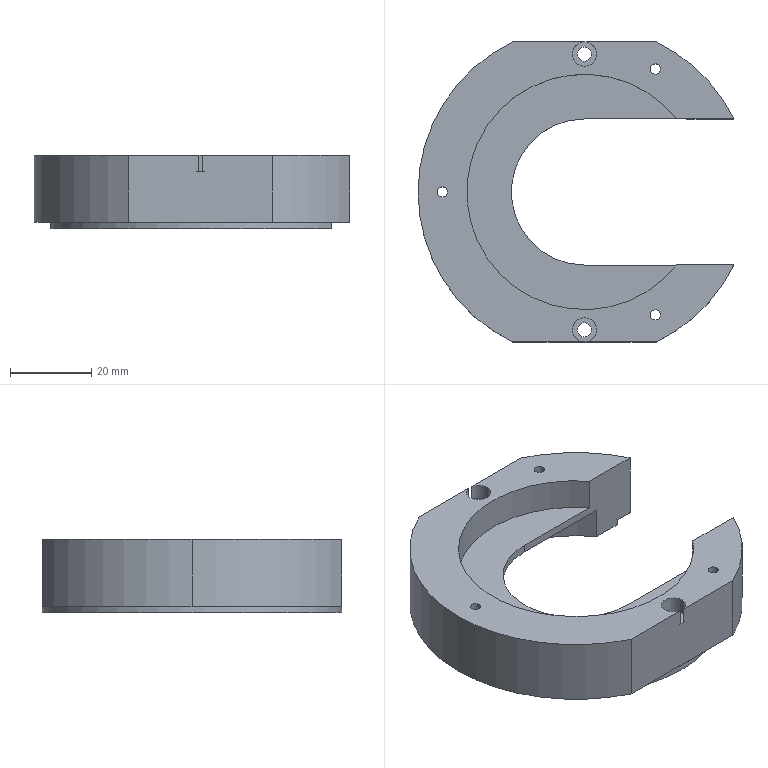Part | SolidWorks | features ICE 5, 3DProfileFeature 2, HoleWzd 2, CirPattern 1, Extrusion 1 | 1 solid | 38 faces | box 77.837 x 73.95 x 18 mm | volume 34057 mm3 | cylinder 25 | plane 13 | commonest cylinder face diameters 2.5 x6 6 x6 3.5 x4 82 x4 62 x2 36 x1
STEP:
#1=CARTESIAN_POINT('',(16.25,30.311,-1.5));
#2=VERTEX_POINT('',#1);
#3=CARTESIAN_POINT('',(18.75,30.311,-1.5));
#4=VERTEX_POINT('',#3);
#5=CARTESIAN_POINT('',(17.5,30.311,-1.5));
#6=DIRECTION('',(0.,0.,1.));
#7=DIRECTION('',(1.,0.,0.));
#8=AXIS2_PLACEMENT_3D('',#5,#6,#7);
#9=CIRCLE('',#8,1.25);
#10=EDGE_CURVE('',#2,#4,#9,.T.);
#11=ORIENTED_EDGE('',*,*,#10,.F.);
#12=CARTESIAN_POINT('',(16.25,30.311,16.5));
#13=VERTEX_POINT('',#12);
#14=CARTESIAN_POINT('',(16.25,30.311,16.5));
#15=DIRECTION('',(0.,0.,1.));
#16=VECTOR('',#15,1000.);
#17=LINE('',#14,#16);
#18=EDGE_CURVE('',#2,#13,#17,.T.);
#19=ORIENTED_EDGE('',*,*,#18,.T.);
#20=CARTESIAN_POINT('',(18.75,30.311,16.5));
#21=VERTEX_POINT('',#20);
#22=CARTESIAN_POINT('',(17.5,30.311,16.5));
#23=DIRECTION('',(0.,0.,1.));
#24=DIRECTION('',(1.,0.,0.));
#25=AXIS2_PLACEMENT_3D('',#22,#23,#24);
#26=CIRCLE('',#25,1.25);
#27=EDGE_CURVE('',#13,#21,#26,.T.);
#28=ORIENTED_EDGE('',*,*,#27,.T.);
#29=CARTESIAN_POINT('',(18.75,30.311,16.5));
#30=DIRECTION('',(0.,0.,1.));
#31=VECTOR('',#30,1000.);
#32=LINE('',#29,#31);
#33=EDGE_CURVE('',#4,#21,#32,.T.);
#34=ORIENTED_EDGE('',*,*,#33,.F.);
#35=EDGE_LOOP('',(#11,#19,#28,#34));
#36=FACE_OUTER_BOUND('',#35,.T.);
#37=CARTESIAN_POINT('',(17.5,30.311,16.5));
#38=DIRECTION('',(0.,0.,1.));
#39=DIRECTION('',(1.,0.,0.));
#40=AXIS2_PLACEMENT_3D('',#37,#38,#39);
#41=CYLINDRICAL_SURFACE('',#40,1.25);
#42=ADVANCED_FACE('',(#36),#41,.F.);
#43=CARTESIAN_POINT('',(16.25,-30.311,-1.5));
#44=VERTEX_POINT('',#43);
#45=CARTESIAN_POINT('',(18.75,-30.311,-1.5));
#46=VERTEX_POINT('',#45);
#47=CARTESIAN_POINT('',(17.5,-30.311,-1.5));
#48=DIRECTION('',(0.,0.,1.));
#49=DIRECTION('',(1.,0.,0.));
#50=AXIS2_PLACEMENT_3D('',#47,#48,#49);
#51=CIRCLE('',#50,1.25);
#52=EDGE_CURVE('',#44,#46,#51,.T.);
#53=ORIENTED_EDGE('',*,*,#52,.F.);
#54=CARTESIAN_POINT('',(16.25,-30.311,16.5));
#55=VERTEX_POINT('',#54);
#56=CARTESIAN_POINT('',(16.25,-30.311,16.5));
#57=DIRECTION('',(0.,0.,1.));
#58=VECTOR('',#57,1000.);
#59=LINE('',#56,#58);
#60=EDGE_CURVE('',#44,#55,#59,.T.);
#61=ORIENTED_EDGE('',*,*,#60,.T.);
#62=CARTESIAN_POINT('',(18.75,-30.311,16.5));
#63=VERTEX_POINT('',#62);
#64=CARTESIAN_POINT('',(17.5,-30.311,16.5));
#65=DIRECTION('',(0.,0.,1.));
#66=DIRECTION('',(1.,0.,0.));
#67=AXIS2_PLACEMENT_3D('',#64,#65,#66);
#68=CIRCLE('',#67,1.25);
#69=EDGE_CURVE('',#55,#63,#68,.T.);
#70=ORIENTED_EDGE('',*,*,#69,.T.);
#71=CARTESIAN_POINT('',(18.75,-30.311,16.5));
#72=DIRECTION('',(0.,0.,1.));
#73=VECTOR('',#72,1000.);
#74=LINE('',#71,#73);
#75=EDGE_CURVE('',#46,#63,#74,.T.);
#76=ORIENTED_EDGE('',*,*,#75,.F.);
#77=EDGE_LOOP('',(#53,#61,#70,#76));
#78=FACE_OUTER_BOUND('',#77,.T.);
#79=CARTESIAN_POINT('',(17.5,-30.311,16.5));
#80=DIRECTION('',(0.,0.,1.));
#81=DIRECTION('',(1.,0.,0.));
#82=AXIS2_PLACEMENT_3D('',#79,#80,#81);
#83=CYLINDRICAL_SURFACE('',#82,1.25);
#84=ADVANCED_FACE('',(#78),#83,.F.);
#85=CARTESIAN_POINT('',(-36.25,0.,-1.5));
#86=VERTEX_POINT('',#85);
#87=CARTESIAN_POINT('',(-33.75,0.,-1.5));
#88=VERTEX_POINT('',#87);
#89=CARTESIAN_POINT('',(-35.,0.,-1.5));
#90=DIRECTION('',(0.,0.,1.));
#91=DIRECTION('',(1.,0.,0.));
#92=AXIS2_PLACEMENT_3D('',#89,#90,#91);
#93=CIRCLE('',#92,1.25);
#94=EDGE_CURVE('',#86,#88,#93,.T.);
#95=ORIENTED_EDGE('',*,*,#94,.F.);
#96=CARTESIAN_POINT('',(-36.25,0.,16.5));
#97=VERTEX_POINT('',#96);
#98=CARTESIAN_POINT('',(-36.25,0.,16.5));
#99=DIRECTION('',(0.,0.,1.));
#100=VECTOR('',#99,1000.);
#101=LINE('',#98,#100);
#102=EDGE_CURVE('',#86,#97,#101,.T.);
#103=ORIENTED_EDGE('',*,*,#102,.T.);
#104=CARTESIAN_POINT('',(-33.75,0.,16.5));
#105=VERTEX_POINT('',#104);
#106=CARTESIAN_POINT('',(-35.,0.,16.5));
#107=DIRECTION('',(0.,0.,1.));
#108=DIRECTION('',(1.,0.,0.));
#109=AXIS2_PLACEMENT_3D('',#106,#107,#108);
#110=CIRCLE('',#109,1.25);
#111=EDGE_CURVE('',#97,#105,#110,.T.);
#112=ORIENTED_EDGE('',*,*,#111,.T.);
#113=CARTESIAN_POINT('',(-33.75,0.,16.5));
#114=DIRECTION('',(0.,0.,1.));
#115=VECTOR('',#114,1000.);
#116=LINE('',#113,#115);
#117=EDGE_CURVE('',#88,#105,#116,.T.);
#118=ORIENTED_EDGE('',*,*,#117,.F.);
#119=EDGE_LOOP('',(#95,#103,#112,#118));
#120=FACE_OUTER_BOUND('',#119,.T.);
#121=CARTESIAN_POINT('',(-35.,0.,16.5));
#122=DIRECTION('',(0.,0.,1.));
#123=DIRECTION('',(1.,0.,0.));
#124=AXIS2_PLACEMENT_3D('',#121,#122,#123);
#125=CYLINDRICAL_SURFACE('',#124,1.25);
#126=ADVANCED_FACE('',(#120),#125,.F.);
#127=CARTESIAN_POINT('',(-1.75,34.,-1.5));
#128=VERTEX_POINT('',#127);
#129=CARTESIAN_POINT('',(1.75,34.,-1.5));
#130=VERTEX_POINT('',#129);
#131=CARTESIAN_POINT('',(0.,34.,-1.5));
#132=DIRECTION('',(0.,0.,1.));
#133=DIRECTION('',(1.,0.,0.));
#134=AXIS2_PLACEMENT_3D('',#131,#132,#133);
#135=CIRCLE('',#134,1.75);
#136=EDGE_CURVE('',#128,#130,#135,.T.);
#137=ORIENTED_EDGE('',*,*,#136,.F.);
#138=CARTESIAN_POINT('',(-1.75,34.,12.5));
#139=VERTEX_POINT('',#138);
#140=CARTESIAN_POINT('',(-1.75,34.,16.5));
#141=DIRECTION('',(0.,0.,1.));
#142=VECTOR('',#141,1000.);
#143=LINE('',#140,#142);
#144=EDGE_CURVE('',#128,#139,#143,.T.);
#145=ORIENTED_EDGE('',*,*,#144,.T.);
#146=CARTESIAN_POINT('',(1.75,34.,12.5));
#147=VERTEX_POINT('',#146);
#148=CARTESIAN_POINT('',(0.,34.,12.5));
#149=DIRECTION('',(0.,0.,1.));
#150=DIRECTION('',(1.,0.,0.));
#151=AXIS2_PLACEMENT_3D('',#148,#149,#150);
#152=CIRCLE('',#151,1.75);
#153=EDGE_CURVE('',#139,#147,#152,.T.);
#154=ORIENTED_EDGE('',*,*,#153,.T.);
#155=CARTESIAN_POINT('',(1.75,34.,16.5));
#156=DIRECTION('',(0.,0.,1.));
#157=VECTOR('',#156,1000.);
#158=LINE('',#155,#157);
#159=EDGE_CURVE('',#130,#147,#158,.T.);
#160=ORIENTED_EDGE('',*,*,#159,.F.);
#161=EDGE_LOOP('',(#137,#145,#154,#160));
#162=FACE_OUTER_BOUND('',#161,.T.);
#163=CARTESIAN_POINT('',(0.,34.,16.5));
#164=DIRECTION('',(0.,0.,1.));
#165=DIRECTION('',(1.,0.,0.));
#166=AXIS2_PLACEMENT_3D('',#163,#164,#165);
#167=CYLINDRICAL_SURFACE('',#166,1.75);
#168=ADVANCED_FACE('',(#162),#167,.F.);
#169=CARTESIAN_POINT('',(-3.,34.,12.5));
#170=VERTEX_POINT('',#169);
#171=CARTESIAN_POINT('',(3.,34.,12.5));
#172=VERTEX_POINT('',#171);
#173=CARTESIAN_POINT('',(0.,34.,12.5));
#174=DIRECTION('',(0.,0.,1.));
#175=DIRECTION('',(1.,0.,0.));
#176=AXIS2_PLACEMENT_3D('',#173,#174,#175);
#177=CIRCLE('',#176,3.);
#178=EDGE_CURVE('',#170,#172,#177,.T.);
#179=ORIENTED_EDGE('',*,*,#178,.F.);
#180=CARTESIAN_POINT('',(-3.,34.,16.5));
#181=VERTEX_POINT('',#180);
#182=CARTESIAN_POINT('',(-3.,34.,16.5));
#183=DIRECTION('',(0.,0.,1.));
#184=VECTOR('',#183,1000.);
#185=LINE('',#182,#184);
#186=EDGE_CURVE('',#170,#181,#185,.T.);
#187=ORIENTED_EDGE('',*,*,#186,.T.);
#188=CARTESIAN_POINT('',(3.,34.,16.5));
#189=VERTEX_POINT('',#188);
#190=CARTESIAN_POINT('',(0.,34.,16.5));
#191=DIRECTION('',(0.,0.,1.));
#192=DIRECTION('',(1.,0.,0.));
#193=AXIS2_PLACEMENT_3D('',#190,#191,#192);
#194=CIRCLE('',#193,3.);
#195=EDGE_CURVE('',#181,#189,#194,.T.);
#196=ORIENTED_EDGE('',*,*,#195,.T.);
#197=CARTESIAN_POINT('',(3.,34.,16.5));
#198=DIRECTION('',(0.,0.,1.));
#199=VECTOR('',#198,1000.);
#200=LINE('',#197,#199);
#201=EDGE_CURVE('',#172,#189,#200,.T.);
#202=ORIENTED_EDGE('',*,*,#201,.F.);
#203=EDGE_LOOP('',(#179,#187,#196,#202));
#204=FACE_OUTER_BOUND('',#203,.T.);
#205=CARTESIAN_POINT('',(0.,34.,16.5));
#206=DIRECTION('',(0.,0.,1.));
#207=DIRECTION('',(1.,0.,0.));
#208=AXIS2_PLACEMENT_3D('',#205,#206,#207);
#209=CYLINDRICAL_SURFACE('',#208,3.);
#210=ADVANCED_FACE('',(#204),#209,.F.);
#211=CARTESIAN_POINT('',(0.3865,36.975,12.5));
#212=VERTEX_POINT('',#211);
#213=CARTESIAN_POINT('',(0.,34.,12.5));
#214=DIRECTION('',(0.,0.,1.));
#215=DIRECTION('',(1.,0.,0.));
#216=AXIS2_PLACEMENT_3D('',#213,#214,#215);
#217=CIRCLE('',#216,3.);
#218=EDGE_CURVE('',#172,#212,#217,.T.);
#219=ORIENTED_EDGE('',*,*,#218,.F.);
#220=ORIENTED_EDGE('',*,*,#201,.T.);
#221=CARTESIAN_POINT('',(0.3865,36.975,16.5));
#222=VERTEX_POINT('',#221);
#223=CARTESIAN_POINT('',(0.,34.,16.5));
#224=DIRECTION('',(0.,0.,1.));
#225=DIRECTION('',(1.,0.,0.));
#226=AXIS2_PLACEMENT_3D('',#223,#224,#225);
#227=CIRCLE('',#226,3.);
#228=EDGE_CURVE('',#189,#222,#227,.T.);
#229=ORIENTED_EDGE('',*,*,#228,.T.);
#230=CARTESIAN_POINT('',(0.3865,36.975,16.5));
#231=DIRECTION('',(0.,0.,1.));
#232=VECTOR('',#231,1000.);
#233=LINE('',#230,#232);
#234=EDGE_CURVE('',#212,#222,#233,.T.);
#235=ORIENTED_EDGE('',*,*,#234,.F.);
#236=EDGE_LOOP('',(#219,#220,#229,#235));
#237=FACE_OUTER_BOUND('',#236,.T.);
#238=CARTESIAN_POINT('',(0.,34.,16.5));
#239=DIRECTION('',(0.,0.,1.));
#240=DIRECTION('',(1.,0.,0.));
#241=AXIS2_PLACEMENT_3D('',#238,#239,#240);
#242=CYLINDRICAL_SURFACE('',#241,3.);
#243=ADVANCED_FACE('',(#237),#242,.F.);
#244=CARTESIAN_POINT('',(-1.75,-34.,-1.5));
#245=VERTEX_POINT('',#244);
#246=CARTESIAN_POINT('',(1.75,-34.,-1.5));
#247=VERTEX_POINT('',#246);
#248=CARTESIAN_POINT('',(0.,-34.,-1.5));
#249=DIRECTION('',(0.,0.,1.));
#250=DIRECTION('',(1.,0.,0.));
#251=AXIS2_PLACEMENT_3D('',#248,#249,#250);
#252=CIRCLE('',#251,1.75);
#253=EDGE_CURVE('',#245,#247,#252,.T.);
#254=ORIENTED_EDGE('',*,*,#253,.F.);
#255=CARTESIAN_POINT('',(-1.75,-34.,12.5));
#256=VERTEX_POINT('',#255);
#257=CARTESIAN_POINT('',(-1.75,-34.,16.5));
#258=DIRECTION('',(0.,0.,1.));
#259=VECTOR('',#258,1000.);
#260=LINE('',#257,#259);
#261=EDGE_CURVE('',#245,#256,#260,.T.);
#262=ORIENTED_EDGE('',*,*,#261,.T.);
#263=CARTESIAN_POINT('',(1.75,-34.,12.5));
#264=VERTEX_POINT('',#263);
#265=CARTESIAN_POINT('',(0.,-34.,12.5));
#266=DIRECTION('',(0.,0.,1.));
#267=DIRECTION('',(1.,0.,0.));
#268=AXIS2_PLACEMENT_3D('',#265,#266,#267);
#269=CIRCLE('',#268,1.75);
#270=EDGE_CURVE('',#256,#264,#269,.T.);
#271=ORIENTED_EDGE('',*,*,#270,.T.);
#272=CARTESIAN_POINT('',(1.75,-34.,16.5));
#273=DIRECTION('',(0.,0.,1.));
#274=VECTOR('',#273,1000.);
#275=LINE('',#272,#274);
#276=EDGE_CURVE('',#247,#264,#275,.T.);
#277=ORIENTED_EDGE('',*,*,#276,.F.);
#278=EDGE_LOOP('',(#254,#262,#271,#277));
#279=FACE_OUTER_BOUND('',#278,.T.);
#280=CARTESIAN_POINT('',(0.,-34.,16.5));
#281=DIRECTION('',(0.,0.,1.));
#282=DIRECTION('',(1.,0.,0.));
#283=AXIS2_PLACEMENT_3D('',#280,#281,#282);
#284=CYLINDRICAL_SURFACE('',#283,1.75);
#285=ADVANCED_FACE('',(#279),#284,.F.);
#286=CARTESIAN_POINT('',(-3.,-34.,12.5));
#287=VERTEX_POINT('',#286);
#288=CARTESIAN_POINT('',(-0.3865,-36.975,12.5));
#289=VERTEX_POINT('',#288);
#290=CARTESIAN_POINT('',(0.,-34.,12.5));
#291=DIRECTION('',(0.,0.,1.));
#292=DIRECTION('',(1.,0.,0.));
#293=AXIS2_PLACEMENT_3D('',#290,#291,#292);
#294=CIRCLE('',#293,3.);
#295=EDGE_CURVE('',#287,#289,#294,.T.);
#296=ORIENTED_EDGE('',*,*,#295,.F.);
#297=CARTESIAN_POINT('',(-3.,-34.,16.5));
#298=VERTEX_POINT('',#297);
#299=CARTESIAN_POINT('',(-3.,-34.,16.5));
#300=DIRECTION('',(0.,0.,1.));
#301=VECTOR('',#300,1000.);
#302=LINE('',#299,#301);
#303=EDGE_CURVE('',#287,#298,#302,.T.);
#304=ORIENTED_EDGE('',*,*,#303,.T.);
#305=CARTESIAN_POINT('',(-0.3865,-36.975,16.5));
#306=VERTEX_POINT('',#305);
#307=CARTESIAN_POINT('',(0.,-34.,16.5));
#308=DIRECTION('',(0.,0.,1.));
#309=DIRECTION('',(1.,0.,0.));
#310=AXIS2_PLACEMENT_3D('',#307,#308,#309);
#311=CIRCLE('',#310,3.);
#312=EDGE_CURVE('',#298,#306,#311,.T.);
#313=ORIENTED_EDGE('',*,*,#312,.T.);
#314=CARTESIAN_POINT('',(-0.3865,-36.975,16.5));
#315=DIRECTION('',(0.,0.,1.));
#316=VECTOR('',#315,1000.);
#317=LINE('',#314,#316);
#318=EDGE_CURVE('',#289,#306,#317,.T.);
#319=ORIENTED_EDGE('',*,*,#318,.F.);
#320=EDGE_LOOP('',(#296,#304,#313,#319));
#321=FACE_OUTER_BOUND('',#320,.T.);
#322=CARTESIAN_POINT('',(0.,-34.,16.5));
#323=DIRECTION('',(0.,0.,1.));
#324=DIRECTION('',(1.,0.,0.));
#325=AXIS2_PLACEMENT_3D('',#322,#323,#324);
#326=CYLINDRICAL_SURFACE('',#325,3.);
#327=ADVANCED_FACE('',(#321),#326,.F.);
#328=ORIENTED_EDGE('',*,*,#303,.F.);
#329=CARTESIAN_POINT('',(3.,-34.,12.5));
#330=VERTEX_POINT('',#329);
#331=CARTESIAN_POINT('',(0.,-34.,12.5));
#332=DIRECTION('',(0.,0.,1.));
#333=DIRECTION('',(1.,0.,0.));
#334=AXIS2_PLACEMENT_3D('',#331,#332,#333);
#335=CIRCLE('',#334,3.);
#336=EDGE_CURVE('',#330,#287,#335,.T.);
#337=ORIENTED_EDGE('',*,*,#336,.F.);
#338=CARTESIAN_POINT('',(3.,-34.,16.5));
#339=VERTEX_POINT('',#338);
#340=CARTESIAN_POINT('',(3.,-34.,16.5));
#341=DIRECTION('',(0.,0.,1.));
#342=VECTOR('',#341,1000.);
#343=LINE('',#340,#342);
#344=EDGE_CURVE('',#330,#339,#343,.T.);
#345=ORIENTED_EDGE('',*,*,#344,.T.);
#346=CARTESIAN_POINT('',(0.,-34.,16.5));
#347=DIRECTION('',(0.,0.,1.));
#348=DIRECTION('',(1.,0.,0.));
#349=AXIS2_PLACEMENT_3D('',#346,#347,#348);
#350=CIRCLE('',#349,3.);
#351=EDGE_CURVE('',#339,#298,#350,.T.);
#352=ORIENTED_EDGE('',*,*,#351,.T.);
#353=EDGE_LOOP('',(#328,#337,#345,#352));
#354=FACE_OUTER_BOUND('',#353,.T.);
#355=CARTESIAN_POINT('',(0.,-34.,16.5));
#356=DIRECTION('',(0.,0.,1.));
#357=DIRECTION('',(1.,0.,0.));
#358=AXIS2_PLACEMENT_3D('',#355,#356,#357);
#359=CYLINDRICAL_SURFACE('',#358,3.);
#360=ADVANCED_FACE('',(#354),#359,.F.);
#361=CARTESIAN_POINT('',(-31.,0.,6.5));
#362=VERTEX_POINT('',#361);
#363=CARTESIAN_POINT('',(25.239,18.,6.5));
#364=VERTEX_POINT('',#363);
#365=CARTESIAN_POINT('',(0.,0.,6.5));
#366=DIRECTION('',(0.,0.,-1.));
#367=DIRECTION('',(-1.,0.,0.));
#368=AXIS2_PLACEMENT_3D('',#365,#366,#367);
#369=CIRCLE('',#368,31.);
#370=EDGE_CURVE('',#362,#364,#369,.T.);
#371=ORIENTED_EDGE('',*,*,#370,.F.);
#372=CARTESIAN_POINT('',(-31.,0.,-1.5));
#373=VERTEX_POINT('',#372);
#374=CARTESIAN_POINT('',(-31.,0.,6.5));
#375=DIRECTION('',(0.,0.,-1.));
#376=VECTOR('',#375,1000.);
#377=LINE('',#374,#376);
#378=EDGE_CURVE('',#362,#373,#377,.T.);
#379=ORIENTED_EDGE('',*,*,#378,.T.);
#380=CARTESIAN_POINT('',(25.239,18.,-1.5));
#381=VERTEX_POINT('',#380);
#382=CARTESIAN_POINT('',(0.,0.,-1.5));
#383=DIRECTION('',(0.,0.,-1.));
#384=DIRECTION('',(-1.,0.,0.));
#385=AXIS2_PLACEMENT_3D('',#382,#383,#384);
#386=CIRCLE('',#385,31.);
#387=EDGE_CURVE('',#373,#381,#386,.T.);
#388=ORIENTED_EDGE('',*,*,#387,.T.);
#389=CARTESIAN_POINT('',(25.239,18.,6.5));
#390=DIRECTION('',(0.,0.,1.));
#391=VECTOR('',#390,1000.);
#392=LINE('',#389,#391);
#393=EDGE_CURVE('',#381,#364,#392,.T.);
#394=ORIENTED_EDGE('',*,*,#393,.T.);
#395=EDGE_LOOP('',(#371,#379,#388,#394));
#396=FACE_OUTER_BOUND('',#395,.T.);
#397=CARTESIAN_POINT('',(0.,0.,6.5));
#398=DIRECTION('',(0.,0.,-1.));
#399=DIRECTION('',(-1.,0.,0.));
#400=AXIS2_PLACEMENT_3D('',#397,#398,#399);
#401=CYLINDRICAL_SURFACE('',#400,31.);
#402=ADVANCED_FACE('',(#396),#401,.F.);
#403=CARTESIAN_POINT('',(-41.,0.,16.5));
#404=VERTEX_POINT('',#403);
#405=CARTESIAN_POINT('',(-17.716,-36.975,16.5));
#406=VERTEX_POINT('',#405);
#407=CARTESIAN_POINT('',(0.,0.,16.5));
#408=DIRECTION('',(0.,0.,1.));
#409=DIRECTION('',(1.,0.,0.));
#410=AXIS2_PLACEMENT_3D('',#407,#408,#409);
#411=CIRCLE('',#410,41.);
#412=EDGE_CURVE('',#404,#406,#411,.T.);
#413=ORIENTED_EDGE('',*,*,#412,.F.);
#414=CARTESIAN_POINT('',(-41.,0.,0.));
#415=VERTEX_POINT('',#414);
#416=CARTESIAN_POINT('',(-41.,0.,16.5));
#417=DIRECTION('',(0.,0.,-1.));
#418=VECTOR('',#417,1000.);
#419=LINE('',#416,#418);
#420=EDGE_CURVE('',#404,#415,#419,.T.);
#421=ORIENTED_EDGE('',*,*,#420,.T.);
#422=CARTESIAN_POINT('',(-17.716,-36.975,0.));
#423=VERTEX_POINT('',#422);
#424=CARTESIAN_POINT('',(0.,0.,0.));
#425=DIRECTION('',(0.,0.,1.));
#426=DIRECTION('',(1.,0.,0.));
#427=AXIS2_PLACEMENT_3D('',#424,#425,#426);
#428=CIRCLE('',#427,41.);
#429=EDGE_CURVE('',#415,#423,#428,.T.);
#430=ORIENTED_EDGE('',*,*,#429,.T.);
#431=CARTESIAN_POINT('',(-17.716,-36.975,16.5));
#432=DIRECTION('',(0.,0.,1.));
#433=VECTOR('',#432,1000.);
#434=LINE('',#431,#433);
#435=EDGE_CURVE('',#423,#406,#434,.T.);
#436=ORIENTED_EDGE('',*,*,#435,.T.);
#437=EDGE_LOOP('',(#413,#421,#430,#436));
#438=FACE_OUTER_BOUND('',#437,.T.);
#439=CARTESIAN_POINT('',(0.,0.,16.5));
#440=DIRECTION('',(0.,0.,-1.));
#441=DIRECTION('',(-1.,0.,0.));
#442=AXIS2_PLACEMENT_3D('',#439,#440,#441);
#443=CYLINDRICAL_SURFACE('',#442,41.);
#444=ADVANCED_FACE('',(#438),#443,.T.);
#445=CARTESIAN_POINT('',(17.5,-30.311,-1.5));
#446=DIRECTION('',(0.,0.,1.));
#447=DIRECTION('',(1.,0.,0.));
#448=AXIS2_PLACEMENT_3D('',#445,#446,#447);
#449=CIRCLE('',#448,1.25);
#450=EDGE_CURVE('',#46,#44,#449,.T.);
#451=ORIENTED_EDGE('',*,*,#450,.T.);
#452=ORIENTED_EDGE('',*,*,#52,.T.);
#453=EDGE_LOOP('',(#451,#452));
#454=FACE_BOUND('',#453,.T.);
#455=CARTESIAN_POINT('',(0.,34.,-1.5));
#456=DIRECTION('',(0.,0.,1.));
#457=DIRECTION('',(1.,0.,0.));
#458=AXIS2_PLACEMENT_3D('',#455,#456,#457);
#459=CIRCLE('',#458,1.75);
#460=EDGE_CURVE('',#130,#128,#459,.T.);
#461=ORIENTED_EDGE('',*,*,#460,.T.);
#462=ORIENTED_EDGE('',*,*,#136,.T.);
#463=EDGE_LOOP('',(#461,#462));
#464=FACE_BOUND('',#463,.T.);
#465=CARTESIAN_POINT('',(0.,-34.,-1.5));
#466=DIRECTION('',(0.,0.,1.));
#467=DIRECTION('',(1.,0.,0.));
#468=AXIS2_PLACEMENT_3D('',#465,#466,#467);
#469=CIRCLE('',#468,1.75);
#470=EDGE_CURVE('',#247,#245,#469,.T.);
#471=ORIENTED_EDGE('',*,*,#470,.T.);
#472=ORIENTED_EDGE('',*,*,#253,.T.);
#473=EDGE_LOOP('',(#471,#472));
#474=FACE_BOUND('',#473,.T.);
#475=CARTESIAN_POINT('',(32.298,18.,-1.5));
#476=VERTEX_POINT('',#475);
#477=CARTESIAN_POINT('',(0.,18.,-1.5));
#478=DIRECTION('',(-1.,0.,0.));
#479=VECTOR('',#478,1000.);
#480=LINE('',#477,#479);
#481=EDGE_CURVE('',#476,#381,#480,.T.);
#482=ORIENTED_EDGE('',*,*,#481,.T.);
#483=ORIENTED_EDGE('',*,*,#387,.F.);
#484=CARTESIAN_POINT('',(25.239,-18.,-1.5));
#485=VERTEX_POINT('',#484);
#486=CARTESIAN_POINT('',(0.,0.,-1.5));
#487=DIRECTION('',(0.,0.,-1.));
#488=DIRECTION('',(-1.,0.,0.));
#489=AXIS2_PLACEMENT_3D('',#486,#487,#488);
#490=CIRCLE('',#489,31.);
#491=EDGE_CURVE('',#485,#373,#490,.T.);
#492=ORIENTED_EDGE('',*,*,#491,.F.);
#493=CARTESIAN_POINT('',(32.298,-18.,-1.5));
#494=VERTEX_POINT('',#493);
#495=CARTESIAN_POINT('',(0.,-18.,-1.5));
#496=DIRECTION('',(1.,0.,0.));
#497=VECTOR('',#496,1000.);
#498=LINE('',#495,#497);
#499=EDGE_CURVE('',#485,#494,#498,.T.);
#500=ORIENTED_EDGE('',*,*,#499,.T.);
#501=CARTESIAN_POINT('',(0.,0.,-1.5));
#502=DIRECTION('',(0.,0.,-1.));
#503=DIRECTION('',(-1.,0.,0.));
#504=AXIS2_PLACEMENT_3D('',#501,#502,#503);
#505=CIRCLE('',#504,36.975);
#506=EDGE_CURVE('',#494,#476,#505,.T.);
#507=ORIENTED_EDGE('',*,*,#506,.T.);
#508=EDGE_LOOP('',(#482,#483,#492,#500,#507));
#509=FACE_OUTER_BOUND('',#508,.T.);
#510=CARTESIAN_POINT('',(-35.,0.,-1.5));
#511=DIRECTION('',(0.,0.,1.));
#512=DIRECTION('',(1.,0.,0.));
#513=AXIS2_PLACEMENT_3D('',#510,#511,#512);
#514=CIRCLE('',#513,1.25);
#515=EDGE_CURVE('',#88,#86,#514,.T.);
#516=ORIENTED_EDGE('',*,*,#515,.T.);
#517=ORIENTED_EDGE('',*,*,#94,.T.);
#518=EDGE_LOOP('',(#516,#517));
#519=FACE_BOUND('',#518,.T.);
#520=CARTESIAN_POINT('',(17.5,30.311,-1.5));
#521=DIRECTION('',(0.,0.,1.));
#522=DIRECTION('',(1.,0.,0.));
#523=AXIS2_PLACEMENT_3D('',#520,#521,#522);
#524=CIRCLE('',#523,1.25);
#525=EDGE_CURVE('',#4,#2,#524,.T.);
#526=ORIENTED_EDGE('',*,*,#525,.T.);
#527=ORIENTED_EDGE('',*,*,#10,.T.);
#528=EDGE_LOOP('',(#526,#527));
#529=FACE_BOUND('',#528,.T.);
#530=CARTESIAN_POINT('',(0.,0.,-1.5));
#531=DIRECTION('',(0.,0.,-1.));
#532=DIRECTION('',(-1.,0.,0.));
#533=AXIS2_PLACEMENT_3D('',#530,#531,#532);
#534=PLANE('',#533);
#535=ADVANCED_FACE('',(#454,#464,#474,#509,#519,#529),#534,.T.);
#536=CARTESIAN_POINT('',(36.837,18.,16.5));
#537=VERTEX_POINT('',#536);
#538=CARTESIAN_POINT('',(17.716,36.975,16.5));
#539=VERTEX_POINT('',#538);
#540=CARTESIAN_POINT('',(0.,0.,16.5));
#541=DIRECTION('',(0.,0.,1.));
#542=DIRECTION('',(1.,0.,0.));
#543=AXIS2_PLACEMENT_3D('',#540,#541,#542);
#544=CIRCLE('',#543,41.);
#545=EDGE_CURVE('',#537,#539,#544,.T.);
#546=ORIENTED_EDGE('',*,*,#545,.F.);
#547=CARTESIAN_POINT('',(36.837,18.,0.));
#548=VERTEX_POINT('',#547);
#549=CARTESIAN_POINT('',(36.837,18.,-1.5));
#550=DIRECTION('',(0.,0.,1.));
#551=VECTOR('',#550,1000.);
#552=LINE('',#549,#551);
#553=EDGE_CURVE('',#548,#537,#552,.T.);
#554=ORIENTED_EDGE('',*,*,#553,.F.);
#555=CARTESIAN_POINT('',(17.716,36.975,0.));
#556=VERTEX_POINT('',#555);
#557=CARTESIAN_POINT('',(0.,0.,0.));
#558=DIRECTION('',(0.,0.,1.));
#559=DIRECTION('',(1.,0.,0.));
#560=AXIS2_PLACEMENT_3D('',#557,#558,#559);
#561=CIRCLE('',#560,41.);
#562=EDGE_CURVE('',#548,#556,#561,.T.);
#563=ORIENTED_EDGE('',*,*,#562,.T.);
#564=CARTESIAN_POINT('',(17.716,36.975,16.5));
#565=DIRECTION('',(0.,0.,1.));
#566=VECTOR('',#565,1000.);
#567=LINE('',#564,#566);
#568=EDGE_CURVE('',#556,#539,#567,.T.);
#569=ORIENTED_EDGE('',*,*,#568,.T.);
#570=EDGE_LOOP('',(#546,#554,#563,#569));
#571=FACE_OUTER_BOUND('',#570,.T.);
#572=CARTESIAN_POINT('',(0.,0.,16.5));
#573=DIRECTION('',(0.,0.,-1.));
#574=DIRECTION('',(-1.,0.,0.));
#575=AXIS2_PLACEMENT_3D('',#572,#573,#574);
#576=CYLINDRICAL_SURFACE('',#575,41.);
#577=ADVANCED_FACE('',(#571),#576,.T.);
#578=ORIENTED_EDGE('',*,*,#562,.F.);
#579=CARTESIAN_POINT('',(32.298,18.,0.));
#580=VERTEX_POINT('',#579);
#581=CARTESIAN_POINT('',(0.,18.,0.));
#582=DIRECTION('',(-1.,0.,0.));
#583=VECTOR('',#582,1000.);
#584=LINE('',#581,#583);
#585=EDGE_CURVE('',#548,#580,#584,.T.);
#586=ORIENTED_EDGE('',*,*,#585,.T.);
#587=CARTESIAN_POINT('',(0.,36.975,0.));
#588=VERTEX_POINT('',#587);
#589=CARTESIAN_POINT('',(0.,0.,0.));
#590=DIRECTION('',(0.,0.,-1.));
#591=DIRECTION('',(-1.,0.,0.));
#592=AXIS2_PLACEMENT_3D('',#589,#590,#591);
#593=CIRCLE('',#592,36.975);
#594=EDGE_CURVE('',#588,#580,#593,.T.);
#595=ORIENTED_EDGE('',*,*,#594,.F.);
#596=CARTESIAN_POINT('',(0.,36.975,0.));
#597=DIRECTION('',(1.,0.,0.));
#598=VECTOR('',#597,1000.);
#599=LINE('',#596,#598);
#600=EDGE_CURVE('',#588,#556,#599,.T.);
#601=ORIENTED_EDGE('',*,*,#600,.T.);
#602=EDGE_LOOP('',(#578,#586,#595,#601));
#603=FACE_OUTER_BOUND('',#602,.T.);
#604=CARTESIAN_POINT('',(0.,0.,0.));
#605=DIRECTION('',(0.,0.,1.));
#606=DIRECTION('',(1.,0.,0.));
#607=AXIS2_PLACEMENT_3D('',#604,#605,#606);
#608=PLANE('',#607);
#609=ADVANCED_FACE('',(#603),#608,.F.);
#610=ORIENTED_EDGE('',*,*,#420,.F.);
#611=CARTESIAN_POINT('',(-17.716,36.975,16.5));
#612=VERTEX_POINT('',#611);
#613=CARTESIAN_POINT('',(0.,0.,16.5));
#614=DIRECTION('',(0.,0.,1.));
#615=DIRECTION('',(1.,0.,0.));
#616=AXIS2_PLACEMENT_3D('',#613,#614,#615);
#617=CIRCLE('',#616,41.);
#618=EDGE_CURVE('',#612,#404,#617,.T.);
#619=ORIENTED_EDGE('',*,*,#618,.F.);
#620=CARTESIAN_POINT('',(-17.716,36.975,0.));
#621=VERTEX_POINT('',#620);
#622=CARTESIAN_POINT('',(-17.716,36.975,16.5));
#623=DIRECTION('',(0.,0.,-1.));
#624=VECTOR('',#623,1000.);
#625=LINE('',#622,#624);
#626=EDGE_CURVE('',#612,#621,#625,.T.);
#627=ORIENTED_EDGE('',*,*,#626,.T.);
#628=CARTESIAN_POINT('',(0.,0.,0.));
#629=DIRECTION('',(0.,0.,1.));
#630=DIRECTION('',(1.,0.,0.));
#631=AXIS2_PLACEMENT_3D('',#628,#629,#630);
#632=CIRCLE('',#631,41.);
#633=EDGE_CURVE('',#621,#415,#632,.T.);
#634=ORIENTED_EDGE('',*,*,#633,.T.);
#635=EDGE_LOOP('',(#610,#619,#627,#634));
#636=FACE_OUTER_BOUND('',#635,.T.);
#637=CARTESIAN_POINT('',(0.,0.,16.5));
#638=DIRECTION('',(0.,0.,-1.));
#639=DIRECTION('',(-1.,0.,0.));
#640=AXIS2_PLACEMENT_3D('',#637,#638,#639);
#641=CYLINDRICAL_SURFACE('',#640,41.);
#642=ADVANCED_FACE('',(#636),#641,.T.);
#643=ORIENTED_EDGE('',*,*,#633,.F.);
#644=CARTESIAN_POINT('',(0.,36.975,0.));
#645=DIRECTION('',(1.,0.,0.));
#646=VECTOR('',#645,1000.);
#647=LINE('',#644,#646);
#648=EDGE_CURVE('',#621,#588,#647,.T.);
#649=ORIENTED_EDGE('',*,*,#648,.T.);
#650=CARTESIAN_POINT('',(0.,-36.975,0.));
#651=VERTEX_POINT('',#650);
#652=CARTESIAN_POINT('',(0.,0.,0.));
#653=DIRECTION('',(0.,0.,-1.));
#654=DIRECTION('',(-1.,0.,0.));
#655=AXIS2_PLACEMENT_3D('',#652,#653,#654);
#656=CIRCLE('',#655,36.975);
#657=EDGE_CURVE('',#651,#588,#656,.T.);
#658=ORIENTED_EDGE('',*,*,#657,.F.);
#659=CARTESIAN_POINT('',(0.,-36.975,0.));
#660=DIRECTION('',(-1.,0.,0.));
#661=VECTOR('',#660,1000.);
#662=LINE('',#659,#661);
#663=EDGE_CURVE('',#651,#423,#662,.T.);
#664=ORIENTED_EDGE('',*,*,#663,.T.);
#665=ORIENTED_EDGE('',*,*,#429,.F.);
#666=EDGE_LOOP('',(#643,#649,#658,#664,#665));
#667=FACE_OUTER_BOUND('',#666,.T.);
#668=CARTESIAN_POINT('',(0.,0.,0.));
#669=DIRECTION('',(0.,0.,1.));
#670=DIRECTION('',(1.,0.,0.));
#671=AXIS2_PLACEMENT_3D('',#668,#669,#670);
#672=PLANE('',#671);
#673=ADVANCED_FACE('',(#667),#672,.F.);
#674=CARTESIAN_POINT('',(17.716,-36.975,0.));
#675=VERTEX_POINT('',#674);
#676=CARTESIAN_POINT('',(36.837,-18.,0.));
#677=VERTEX_POINT('',#676);
#678=CARTESIAN_POINT('',(0.,0.,0.));
#679=DIRECTION('',(0.,0.,1.));
#680=DIRECTION('',(1.,0.,0.));
#681=AXIS2_PLACEMENT_3D('',#678,#679,#680);
#682=CIRCLE('',#681,41.);
#683=EDGE_CURVE('',#675,#677,#682,.T.);
#684=ORIENTED_EDGE('',*,*,#683,.T.);
#685=CARTESIAN_POINT('',(36.837,-18.,16.5));
#686=VERTEX_POINT('',#685);
#687=CARTESIAN_POINT('',(36.837,-18.,-1.5));
#688=DIRECTION('',(0.,0.,1.));
#689=VECTOR('',#688,1000.);
#690=LINE('',#687,#689);
#691=EDGE_CURVE('',#677,#686,#690,.T.);
#692=ORIENTED_EDGE('',*,*,#691,.T.);
#693=CARTESIAN_POINT('',(17.716,-36.975,16.5));
#694=VERTEX_POINT('',#693);
#695=CARTESIAN_POINT('',(0.,0.,16.5));
#696=DIRECTION('',(0.,0.,1.));
#697=DIRECTION('',(1.,0.,0.));
#698=AXIS2_PLACEMENT_3D('',#695,#696,#697);
#699=CIRCLE('',#698,41.);
#700=EDGE_CURVE('',#694,#686,#699,.T.);
#701=ORIENTED_EDGE('',*,*,#700,.F.);
#702=CARTESIAN_POINT('',(17.716,-36.975,16.5));
#703=DIRECTION('',(0.,0.,-1.));
#704=VECTOR('',#703,1000.);
#705=LINE('',#702,#704);
#706=EDGE_CURVE('',#694,#675,#705,.T.);
#707=ORIENTED_EDGE('',*,*,#706,.T.);
#708=EDGE_LOOP('',(#684,#692,#701,#707));
#709=FACE_OUTER_BOUND('',#708,.T.);
#710=CARTESIAN_POINT('',(0.,0.,16.5));
#711=DIRECTION('',(0.,0.,-1.));
#712=DIRECTION('',(-1.,0.,0.));
#713=AXIS2_PLACEMENT_3D('',#710,#711,#712);
#714=CYLINDRICAL_SURFACE('',#713,41.);
#715=ADVANCED_FACE('',(#709),#714,.T.);
#716=CARTESIAN_POINT('',(17.5,30.311,16.5));
#717=DIRECTION('',(0.,0.,1.));
#718=DIRECTION('',(1.,0.,0.));
#719=AXIS2_PLACEMENT_3D('',#716,#717,#718);
#720=CIRCLE('',#719,1.25);
#721=EDGE_CURVE('',#21,#13,#720,.T.);
#722=ORIENTED_EDGE('',*,*,#721,.F.);
#723=ORIENTED_EDGE('',*,*,#27,.F.);
#724=EDGE_LOOP('',(#722,#723));
#725=FACE_BOUND('',#724,.T.);
#726=CARTESIAN_POINT('',(17.5,-30.311,16.5));
#727=DIRECTION('',(0.,0.,1.));
#728=DIRECTION('',(1.,0.,0.));
#729=AXIS2_PLACEMENT_3D('',#726,#727,#728);
#730=CIRCLE('',#729,1.25);
#731=EDGE_CURVE('',#63,#55,#730,.T.);
#732=ORIENTED_EDGE('',*,*,#731,.F.);
#733=ORIENTED_EDGE('',*,*,#69,.F.);
#734=EDGE_LOOP('',(#732,#733));
#735=FACE_BOUND('',#734,.T.);
#736=CARTESIAN_POINT('',(-35.,0.,16.5));
#737=DIRECTION('',(0.,0.,1.));
#738=DIRECTION('',(1.,0.,0.));
#739=AXIS2_PLACEMENT_3D('',#736,#737,#738);
#740=CIRCLE('',#739,1.25);
#741=EDGE_CURVE('',#105,#97,#740,.T.);
#742=ORIENTED_EDGE('',*,*,#741,.F.);
#743=ORIENTED_EDGE('',*,*,#111,.F.);
#744=EDGE_LOOP('',(#742,#743));
#745=FACE_BOUND('',#744,.T.);
#746=CARTESIAN_POINT('',(-0.3865,36.975,16.5));
#747=VERTEX_POINT('',#746);
#748=CARTESIAN_POINT('',(0.,34.,16.5));
#749=DIRECTION('',(0.,0.,1.));
#750=DIRECTION('',(1.,0.,0.));
#751=AXIS2_PLACEMENT_3D('',#748,#749,#750);
#752=CIRCLE('',#751,3.);
#753=EDGE_CURVE('',#747,#181,#752,.T.);
#754=ORIENTED_EDGE('',*,*,#753,.F.);
#755=CARTESIAN_POINT('',(25.,36.975,16.5));
#756=DIRECTION('',(-1.,0.,0.));
#757=VECTOR('',#756,1000.);
#758=LINE('',#755,#757);
#759=EDGE_CURVE('',#747,#612,#758,.T.);
#760=ORIENTED_EDGE('',*,*,#759,.T.);
#761=ORIENTED_EDGE('',*,*,#618,.T.);
#762=ORIENTED_EDGE('',*,*,#412,.T.);
#763=CARTESIAN_POINT('',(25.,-36.975,16.5));
#764=DIRECTION('',(1.,0.,0.));
#765=VECTOR('',#764,1000.);
#766=LINE('',#763,#765);
#767=EDGE_CURVE('',#406,#306,#766,.T.);
#768=ORIENTED_EDGE('',*,*,#767,.T.);
#769=ORIENTED_EDGE('',*,*,#312,.F.);
#770=ORIENTED_EDGE('',*,*,#351,.F.);
#771=CARTESIAN_POINT('',(0.3865,-36.975,16.5));
#772=VERTEX_POINT('',#771);
#773=CARTESIAN_POINT('',(0.,-34.,16.5));
#774=DIRECTION('',(0.,0.,1.));
#775=DIRECTION('',(1.,0.,0.));
#776=AXIS2_PLACEMENT_3D('',#773,#774,#775);
#777=CIRCLE('',#776,3.);
#778=EDGE_CURVE('',#772,#339,#777,.T.);
#779=ORIENTED_EDGE('',*,*,#778,.F.);
#780=CARTESIAN_POINT('',(25.,-36.975,16.5));
#781=DIRECTION('',(1.,0.,0.));
#782=VECTOR('',#781,1000.);
#783=LINE('',#780,#782);
#784=EDGE_CURVE('',#772,#694,#783,.T.);
#785=ORIENTED_EDGE('',*,*,#784,.T.);
#786=ORIENTED_EDGE('',*,*,#700,.T.);
#787=CARTESIAN_POINT('',(22.738,-18.,16.5));
#788=VERTEX_POINT('',#787);
#789=CARTESIAN_POINT('',(0.,-18.,16.5));
#790=DIRECTION('',(1.,0.,0.));
#791=VECTOR('',#790,1000.);
#792=LINE('',#789,#791);
#793=EDGE_CURVE('',#788,#686,#792,.T.);
#794=ORIENTED_EDGE('',*,*,#793,.F.);
#795=CARTESIAN_POINT('',(22.738,18.,16.5));
#796=VERTEX_POINT('',#795);
#797=CARTESIAN_POINT('',(0.,0.,16.5));
#798=DIRECTION('',(0.,0.,1.));
#799=DIRECTION('',(1.,0.,0.));
#800=AXIS2_PLACEMENT_3D('',#797,#798,#799);
#801=CIRCLE('',#800,29.);
#802=EDGE_CURVE('',#796,#788,#801,.T.);
#803=ORIENTED_EDGE('',*,*,#802,.F.);
#804=CARTESIAN_POINT('',(0.,18.,16.5));
#805=DIRECTION('',(-1.,0.,0.));
#806=VECTOR('',#805,1000.);
#807=LINE('',#804,#806);
#808=EDGE_CURVE('',#537,#796,#807,.T.);
#809=ORIENTED_EDGE('',*,*,#808,.F.);
#810=ORIENTED_EDGE('',*,*,#545,.T.);
#811=CARTESIAN_POINT('',(25.,36.975,16.5));
#812=DIRECTION('',(-1.,0.,0.));
#813=VECTOR('',#812,1000.);
#814=LINE('',#811,#813);
#815=EDGE_CURVE('',#539,#222,#814,.T.);
#816=ORIENTED_EDGE('',*,*,#815,.T.);
#817=ORIENTED_EDGE('',*,*,#228,.F.);
#818=ORIENTED_EDGE('',*,*,#195,.F.);
#819=EDGE_LOOP('',(#754,#760,#761,#762,#768,#769,#770,#779,#785,#786,#794,#803,#809,#810,#816,#817,#818));
#820=FACE_OUTER_BOUND('',#819,.T.);
#821=CARTESIAN_POINT('',(0.,0.,16.5));
#822=DIRECTION('',(0.,0.,1.));
#823=DIRECTION('',(1.,0.,0.));
#824=AXIS2_PLACEMENT_3D('',#821,#822,#823);
#825=PLANE('',#824);
#826=ADVANCED_FACE('',(#725,#735,#745,#820),#825,.T.);
#827=CARTESIAN_POINT('',(32.298,-18.,0.));
#828=VERTEX_POINT('',#827);
#829=CARTESIAN_POINT('',(0.,0.,0.));
#830=DIRECTION('',(0.,0.,-1.));
#831=DIRECTION('',(-1.,0.,0.));
#832=AXIS2_PLACEMENT_3D('',#829,#830,#831);
#833=CIRCLE('',#832,36.975);
#834=EDGE_CURVE('',#828,#651,#833,.T.);
#835=ORIENTED_EDGE('',*,*,#834,.F.);
#836=CARTESIAN_POINT('',(0.,-18.,0.));
#837=DIRECTION('',(1.,0.,0.));
#838=VECTOR('',#837,1000.);
#839=LINE('',#836,#838);
#840=EDGE_CURVE('',#828,#677,#839,.T.);
#841=ORIENTED_EDGE('',*,*,#840,.T.);
#842=ORIENTED_EDGE('',*,*,#683,.F.);
#843=CARTESIAN_POINT('',(0.,-36.975,0.));
#844=DIRECTION('',(-1.,0.,0.));
#845=VECTOR('',#844,1000.);
#846=LINE('',#843,#845);
#847=EDGE_CURVE('',#675,#651,#846,.T.);
#848=ORIENTED_EDGE('',*,*,#847,.T.);
#849=EDGE_LOOP('',(#835,#841,#842,#848));
#850=FACE_OUTER_BOUND('',#849,.T.);
#851=CARTESIAN_POINT('',(0.,0.,0.));
#852=DIRECTION('',(0.,0.,1.));
#853=DIRECTION('',(1.,0.,0.));
#854=AXIS2_PLACEMENT_3D('',#851,#852,#853);
#855=PLANE('',#854);
#856=ADVANCED_FACE('',(#850),#855,.F.);
#857=ORIENTED_EDGE('',*,*,#594,.T.);
#858=CARTESIAN_POINT('',(32.298,18.,-1.5));
#859=DIRECTION('',(0.,0.,-1.));
#860=VECTOR('',#859,1000.);
#861=LINE('',#858,#860);
#862=EDGE_CURVE('',#580,#476,#861,.T.);
#863=ORIENTED_EDGE('',*,*,#862,.T.);
#864=ORIENTED_EDGE('',*,*,#506,.F.);
#865=CARTESIAN_POINT('',(32.298,-18.,-1.5));
#866=DIRECTION('',(0.,0.,1.));
#867=VECTOR('',#866,1000.);
#868=LINE('',#865,#867);
#869=EDGE_CURVE('',#494,#828,#868,.T.);
#870=ORIENTED_EDGE('',*,*,#869,.T.);
#871=ORIENTED_EDGE('',*,*,#834,.T.);
#872=ORIENTED_EDGE('',*,*,#657,.T.);
#873=EDGE_LOOP('',(#857,#863,#864,#870,#871,#872));
#874=FACE_OUTER_BOUND('',#873,.T.);
#875=CARTESIAN_POINT('',(0.,0.,-1.5));
#876=DIRECTION('',(0.,0.,1.));
#877=DIRECTION('',(1.,0.,0.));
#878=AXIS2_PLACEMENT_3D('',#875,#876,#877);
#879=CYLINDRICAL_SURFACE('',#878,36.975);
#880=ADVANCED_FACE('',(#874),#879,.T.);
#881=CARTESIAN_POINT('',(0.3865,-36.975,12.5));
#882=VERTEX_POINT('',#881);
#883=CARTESIAN_POINT('',(25.,-36.975,12.5));
#884=DIRECTION('',(-1.,0.,0.));
#885=VECTOR('',#884,1000.);
#886=LINE('',#883,#885);
#887=EDGE_CURVE('',#882,#289,#886,.T.);
#888=ORIENTED_EDGE('',*,*,#887,.T.);
#889=ORIENTED_EDGE('',*,*,#318,.T.);
#890=ORIENTED_EDGE('',*,*,#767,.F.);
#891=ORIENTED_EDGE('',*,*,#435,.F.);
#892=ORIENTED_EDGE('',*,*,#663,.F.);
#893=ORIENTED_EDGE('',*,*,#847,.F.);
#894=ORIENTED_EDGE('',*,*,#706,.F.);
#895=ORIENTED_EDGE('',*,*,#784,.F.);
#896=CARTESIAN_POINT('',(0.3865,-36.975,16.5));
#897=DIRECTION('',(0.,0.,-1.));
#898=VECTOR('',#897,1000.);
#899=LINE('',#896,#898);
#900=EDGE_CURVE('',#772,#882,#899,.T.);
#901=ORIENTED_EDGE('',*,*,#900,.T.);
#902=EDGE_LOOP('',(#888,#889,#890,#891,#892,#893,#894,#895,#901));
#903=FACE_OUTER_BOUND('',#902,.T.);
#904=CARTESIAN_POINT('',(25.,-36.975,16.5));
#905=DIRECTION('',(0.,1.,0.));
#906=DIRECTION('',(0.,0.,1.));
#907=AXIS2_PLACEMENT_3D('',#904,#905,#906);
#908=PLANE('',#907);
#909=ADVANCED_FACE('',(#903),#908,.F.);
#910=CARTESIAN_POINT('',(-0.3865,36.975,12.5));
#911=VERTEX_POINT('',#910);
#912=CARTESIAN_POINT('',(25.,36.975,12.5));
#913=DIRECTION('',(1.,0.,0.));
#914=VECTOR('',#913,1000.);
#915=LINE('',#912,#914);
#916=EDGE_CURVE('',#911,#212,#915,.T.);
#917=ORIENTED_EDGE('',*,*,#916,.T.);
#918=ORIENTED_EDGE('',*,*,#234,.T.);
#919=ORIENTED_EDGE('',*,*,#815,.F.);
#920=ORIENTED_EDGE('',*,*,#568,.F.);
#921=ORIENTED_EDGE('',*,*,#600,.F.);
#922=ORIENTED_EDGE('',*,*,#648,.F.);
#923=ORIENTED_EDGE('',*,*,#626,.F.);
#924=ORIENTED_EDGE('',*,*,#759,.F.);
#925=CARTESIAN_POINT('',(-0.3865,36.975,16.5));
#926=DIRECTION('',(0.,0.,-1.));
#927=VECTOR('',#926,1000.);
#928=LINE('',#925,#927);
#929=EDGE_CURVE('',#747,#911,#928,.T.);
#930=ORIENTED_EDGE('',*,*,#929,.T.);
#931=EDGE_LOOP('',(#917,#918,#919,#920,#921,#922,#923,#924,#930));
#932=FACE_OUTER_BOUND('',#931,.T.);
#933=CARTESIAN_POINT('',(25.,36.975,16.5));
#934=DIRECTION('',(0.,-1.,0.));
#935=DIRECTION('',(0.,0.,-1.));
#936=AXIS2_PLACEMENT_3D('',#933,#934,#935);
#937=PLANE('',#936);
#938=ADVANCED_FACE('',(#932),#937,.F.);
#939=ORIENTED_EDGE('',*,*,#378,.F.);
#940=CARTESIAN_POINT('',(25.239,-18.,6.5));
#941=VERTEX_POINT('',#940);
#942=CARTESIAN_POINT('',(0.,0.,6.5));
#943=DIRECTION('',(0.,0.,-1.));
#944=DIRECTION('',(-1.,0.,0.));
#945=AXIS2_PLACEMENT_3D('',#942,#943,#944);
#946=CIRCLE('',#945,31.);
#947=EDGE_CURVE('',#941,#362,#946,.T.);
#948=ORIENTED_EDGE('',*,*,#947,.F.);
#949=CARTESIAN_POINT('',(25.239,-18.,6.5));
#950=DIRECTION('',(0.,0.,-1.));
#951=VECTOR('',#950,1000.);
#952=LINE('',#949,#951);
#953=EDGE_CURVE('',#941,#485,#952,.T.);
#954=ORIENTED_EDGE('',*,*,#953,.T.);
#955=ORIENTED_EDGE('',*,*,#491,.T.);
#956=EDGE_LOOP('',(#939,#948,#954,#955));
#957=FACE_OUTER_BOUND('',#956,.T.);
#958=CARTESIAN_POINT('',(0.,0.,6.5));
#959=DIRECTION('',(0.,0.,-1.));
#960=DIRECTION('',(-1.,0.,0.));
#961=AXIS2_PLACEMENT_3D('',#958,#959,#960);
#962=CYLINDRICAL_SURFACE('',#961,31.);
#963=ADVANCED_FACE('',(#957),#962,.F.);
#964=CARTESIAN_POINT('',(0.,18.,6.5));
#965=VERTEX_POINT('',#964);
#966=CARTESIAN_POINT('',(0.,18.,6.5));
#967=DIRECTION('',(1.,0.,0.));
#968=VECTOR('',#967,1000.);
#969=LINE('',#966,#968);
#970=EDGE_CURVE('',#965,#364,#969,.T.);
#971=ORIENTED_EDGE('',*,*,#970,.F.);
#972=CARTESIAN_POINT('',(0.,-18.,6.5));
#973=VERTEX_POINT('',#972);
#974=CARTESIAN_POINT('',(0.,0.,6.5));
#975=DIRECTION('',(0.,0.,-1.));
#976=DIRECTION('',(-1.,0.,0.));
#977=AXIS2_PLACEMENT_3D('',#974,#975,#976);
#978=CIRCLE('',#977,18.);
#979=EDGE_CURVE('',#973,#965,#978,.T.);
#980=ORIENTED_EDGE('',*,*,#979,.F.);
#981=CARTESIAN_POINT('',(0.,-18.,6.5));
#982=DIRECTION('',(-1.,0.,0.));
#983=VECTOR('',#982,1000.);
#984=LINE('',#981,#983);
#985=EDGE_CURVE('',#941,#973,#984,.T.);
#986=ORIENTED_EDGE('',*,*,#985,.F.);
#987=ORIENTED_EDGE('',*,*,#947,.T.);
#988=ORIENTED_EDGE('',*,*,#370,.T.);
#989=EDGE_LOOP('',(#971,#980,#986,#987,#988));
#990=FACE_OUTER_BOUND('',#989,.T.);
#991=CARTESIAN_POINT('',(0.,0.,6.5));
#992=DIRECTION('',(0.,0.,-1.));
#993=DIRECTION('',(-1.,0.,0.));
#994=AXIS2_PLACEMENT_3D('',#991,#992,#993);
#995=PLANE('',#994);
#996=ADVANCED_FACE('',(#990),#995,.T.);
#997=CARTESIAN_POINT('',(22.738,18.,8.5));
#998=VERTEX_POINT('',#997);
#999=CARTESIAN_POINT('',(22.738,-18.,8.5));
#1000=VERTEX_POINT('',#999);
#1001=CARTESIAN_POINT('',(0.,0.,8.5));
#1002=DIRECTION('',(0.,0.,1.));
#1003=DIRECTION('',(1.,0.,0.));
#1004=AXIS2_PLACEMENT_3D('',#1001,#1002,#1003);
#1005=CIRCLE('',#1004,29.);
#1006=EDGE_CURVE('',#998,#1000,#1005,.T.);
#1007=ORIENTED_EDGE('',*,*,#1006,.F.);
#1008=CARTESIAN_POINT('',(22.738,18.,8.5));
#1009=DIRECTION('',(0.,0.,1.));
#1010=VECTOR('',#1009,1000.);
#1011=LINE('',#1008,#1010);
#1012=EDGE_CURVE('',#998,#796,#1011,.T.);
#1013=ORIENTED_EDGE('',*,*,#1012,.T.);
#1014=ORIENTED_EDGE('',*,*,#802,.T.);
#1015=CARTESIAN_POINT('',(22.738,-18.,8.5));
#1016=DIRECTION('',(0.,0.,-1.));
#1017=VECTOR('',#1016,1000.);
#1018=LINE('',#1015,#1017);
#1019=EDGE_CURVE('',#788,#1000,#1018,.T.);
#1020=ORIENTED_EDGE('',*,*,#1019,.T.);
#1021=EDGE_LOOP('',(#1007,#1013,#1014,#1020));
#1022=FACE_OUTER_BOUND('',#1021,.T.);
#1023=CARTESIAN_POINT('',(0.,0.,8.5));
#1024=DIRECTION('',(0.,0.,1.));
#1025=DIRECTION('',(1.,0.,0.));
#1026=AXIS2_PLACEMENT_3D('',#1023,#1024,#1025);
#1027=CYLINDRICAL_SURFACE('',#1026,29.);
#1028=ADVANCED_FACE('',(#1022),#1027,.F.);
#1029=CARTESIAN_POINT('',(0.,18.,8.5));
#1030=VERTEX_POINT('',#1029);
#1031=CARTESIAN_POINT('',(0.,18.,8.5));
#1032=DIRECTION('',(-1.,0.,0.));
#1033=VECTOR('',#1032,1000.);
#1034=LINE('',#1031,#1033);
#1035=EDGE_CURVE('',#998,#1030,#1034,.T.);
#1036=ORIENTED_EDGE('',*,*,#1035,.F.);
#1037=ORIENTED_EDGE('',*,*,#1006,.T.);
#1038=CARTESIAN_POINT('',(0.,-18.,8.5));
#1039=VERTEX_POINT('',#1038);
#1040=CARTESIAN_POINT('',(0.,-18.,8.5));
#1041=DIRECTION('',(1.,0.,0.));
#1042=VECTOR('',#1041,1000.);
#1043=LINE('',#1040,#1042);
#1044=EDGE_CURVE('',#1039,#1000,#1043,.T.);
#1045=ORIENTED_EDGE('',*,*,#1044,.F.);
#1046=CARTESIAN_POINT('',(0.,0.,8.5));
#1047=DIRECTION('',(0.,0.,1.));
#1048=DIRECTION('',(1.,0.,0.));
#1049=AXIS2_PLACEMENT_3D('',#1046,#1047,#1048);
#1050=CIRCLE('',#1049,18.);
#1051=EDGE_CURVE('',#1030,#1039,#1050,.T.);
#1052=ORIENTED_EDGE('',*,*,#1051,.F.);
#1053=EDGE_LOOP('',(#1036,#1037,#1045,#1052));
#1054=FACE_OUTER_BOUND('',#1053,.T.);
#1055=CARTESIAN_POINT('',(0.,0.,8.5));
#1056=DIRECTION('',(0.,0.,1.));
#1057=DIRECTION('',(1.,0.,0.));
#1058=AXIS2_PLACEMENT_3D('',#1055,#1056,#1057);
#1059=PLANE('',#1058);
#1060=ADVANCED_FACE('',(#1054),#1059,.T.);
#1061=ORIENTED_EDGE('',*,*,#553,.T.);
#1062=ORIENTED_EDGE('',*,*,#808,.T.);
#1063=ORIENTED_EDGE('',*,*,#1012,.F.);
#1064=ORIENTED_EDGE('',*,*,#1035,.T.);
#1065=CARTESIAN_POINT('',(0.,18.,-1.5));
#1066=DIRECTION('',(0.,0.,1.));
#1067=VECTOR('',#1066,1000.);
#1068=LINE('',#1065,#1067);
#1069=EDGE_CURVE('',#965,#1030,#1068,.T.);
#1070=ORIENTED_EDGE('',*,*,#1069,.F.);
#1071=ORIENTED_EDGE('',*,*,#970,.T.);
#1072=ORIENTED_EDGE('',*,*,#393,.F.);
#1073=ORIENTED_EDGE('',*,*,#481,.F.);
#1074=ORIENTED_EDGE('',*,*,#862,.F.);
#1075=ORIENTED_EDGE('',*,*,#585,.F.);
#1076=EDGE_LOOP('',(#1061,#1062,#1063,#1064,#1070,#1071,#1072,#1073,#1074,#1075));
#1077=FACE_OUTER_BOUND('',#1076,.T.);
#1078=CARTESIAN_POINT('',(0.,18.,-1.5));
#1079=DIRECTION('',(0.,1.,0.));
#1080=DIRECTION('',(0.,0.,1.));
#1081=AXIS2_PLACEMENT_3D('',#1078,#1079,#1080);
#1082=PLANE('',#1081);
#1083=ADVANCED_FACE('',(#1077),#1082,.F.);
#1084=ORIENTED_EDGE('',*,*,#869,.F.);
#1085=ORIENTED_EDGE('',*,*,#499,.F.);
#1086=ORIENTED_EDGE('',*,*,#953,.F.);
#1087=ORIENTED_EDGE('',*,*,#985,.T.);
#1088=CARTESIAN_POINT('',(0.,-18.,-1.5));
#1089=DIRECTION('',(0.,0.,1.));
#1090=VECTOR('',#1089,1000.);
#1091=LINE('',#1088,#1090);
#1092=EDGE_CURVE('',#973,#1039,#1091,.T.);
#1093=ORIENTED_EDGE('',*,*,#1092,.T.);
#1094=ORIENTED_EDGE('',*,*,#1044,.T.);
#1095=ORIENTED_EDGE('',*,*,#1019,.F.);
#1096=ORIENTED_EDGE('',*,*,#793,.T.);
#1097=ORIENTED_EDGE('',*,*,#691,.F.);
#1098=ORIENTED_EDGE('',*,*,#840,.F.);
#1099=EDGE_LOOP('',(#1084,#1085,#1086,#1087,#1093,#1094,#1095,#1096,#1097,#1098));
#1100=FACE_OUTER_BOUND('',#1099,.T.);
#1101=CARTESIAN_POINT('',(0.,-18.,-1.5));
#1102=DIRECTION('',(0.,-1.,0.));
#1103=DIRECTION('',(0.,0.,-1.));
#1104=AXIS2_PLACEMENT_3D('',#1101,#1102,#1103);
#1105=PLANE('',#1104);
#1106=ADVANCED_FACE('',(#1100),#1105,.F.);
#1107=ORIENTED_EDGE('',*,*,#979,.T.);
#1108=ORIENTED_EDGE('',*,*,#1069,.T.);
#1109=ORIENTED_EDGE('',*,*,#1051,.T.);
#1110=ORIENTED_EDGE('',*,*,#1092,.F.);
#1111=EDGE_LOOP('',(#1107,#1108,#1109,#1110));
#1112=FACE_OUTER_BOUND('',#1111,.T.);
#1113=CARTESIAN_POINT('',(0.,0.,-1.5));
#1114=DIRECTION('',(0.,0.,1.));
#1115=DIRECTION('',(1.,0.,0.));
#1116=AXIS2_PLACEMENT_3D('',#1113,#1114,#1115);
#1117=CYLINDRICAL_SURFACE('',#1116,18.);
#1118=ADVANCED_FACE('',(#1112),#1117,.F.);
#1119=ORIENTED_EDGE('',*,*,#344,.F.);
#1120=CARTESIAN_POINT('',(0.,-34.,12.5));
#1121=DIRECTION('',(0.,0.,1.));
#1122=DIRECTION('',(1.,0.,0.));
#1123=AXIS2_PLACEMENT_3D('',#1120,#1121,#1122);
#1124=CIRCLE('',#1123,3.);
#1125=EDGE_CURVE('',#882,#330,#1124,.T.);
#1126=ORIENTED_EDGE('',*,*,#1125,.F.);
#1127=ORIENTED_EDGE('',*,*,#900,.F.);
#1128=ORIENTED_EDGE('',*,*,#778,.T.);
#1129=EDGE_LOOP('',(#1119,#1126,#1127,#1128));
#1130=FACE_OUTER_BOUND('',#1129,.T.);
#1131=CARTESIAN_POINT('',(0.,-34.,16.5));
#1132=DIRECTION('',(0.,0.,1.));
#1133=DIRECTION('',(1.,0.,0.));
#1134=AXIS2_PLACEMENT_3D('',#1131,#1132,#1133);
#1135=CYLINDRICAL_SURFACE('',#1134,3.);
#1136=ADVANCED_FACE('',(#1130),#1135,.F.);
#1137=CARTESIAN_POINT('',(0.,-34.,12.5));
#1138=DIRECTION('',(0.,0.,1.));
#1139=DIRECTION('',(1.,0.,0.));
#1140=AXIS2_PLACEMENT_3D('',#1137,#1138,#1139);
#1141=CIRCLE('',#1140,1.75);
#1142=EDGE_CURVE('',#264,#256,#1141,.T.);
#1143=ORIENTED_EDGE('',*,*,#1142,.F.);
#1144=ORIENTED_EDGE('',*,*,#270,.F.);
#1145=EDGE_LOOP('',(#1143,#1144));
#1146=FACE_BOUND('',#1145,.T.);
#1147=ORIENTED_EDGE('',*,*,#1125,.T.);
#1148=ORIENTED_EDGE('',*,*,#336,.T.);
#1149=ORIENTED_EDGE('',*,*,#295,.T.);
#1150=ORIENTED_EDGE('',*,*,#887,.F.);
#1151=EDGE_LOOP('',(#1147,#1148,#1149,#1150));
#1152=FACE_OUTER_BOUND('',#1151,.T.);
#1153=CARTESIAN_POINT('',(1.75,-34.,12.5));
#1154=DIRECTION('',(0.,0.,-1.));
#1155=DIRECTION('',(-1.,0.,0.));
#1156=AXIS2_PLACEMENT_3D('',#1153,#1154,#1155);
#1157=PLANE('',#1156);
#1158=ADVANCED_FACE('',(#1146,#1152),#1157,.F.);
#1159=ORIENTED_EDGE('',*,*,#261,.F.);
#1160=ORIENTED_EDGE('',*,*,#470,.F.);
#1161=ORIENTED_EDGE('',*,*,#276,.T.);
#1162=ORIENTED_EDGE('',*,*,#1142,.T.);
#1163=EDGE_LOOP('',(#1159,#1160,#1161,#1162));
#1164=FACE_OUTER_BOUND('',#1163,.T.);
#1165=CARTESIAN_POINT('',(0.,-34.,16.5));
#1166=DIRECTION('',(0.,0.,1.));
#1167=DIRECTION('',(1.,0.,0.));
#1168=AXIS2_PLACEMENT_3D('',#1165,#1166,#1167);
#1169=CYLINDRICAL_SURFACE('',#1168,1.75);
#1170=ADVANCED_FACE('',(#1164),#1169,.F.);
#1171=CARTESIAN_POINT('',(0.,34.,12.5));
#1172=DIRECTION('',(0.,0.,1.));
#1173=DIRECTION('',(1.,0.,0.));
#1174=AXIS2_PLACEMENT_3D('',#1171,#1172,#1173);
#1175=CIRCLE('',#1174,1.75);
#1176=EDGE_CURVE('',#147,#139,#1175,.T.);
#1177=ORIENTED_EDGE('',*,*,#1176,.F.);
#1178=ORIENTED_EDGE('',*,*,#153,.F.);
#1179=EDGE_LOOP('',(#1177,#1178));
#1180=FACE_BOUND('',#1179,.T.);
#1181=CARTESIAN_POINT('',(0.,34.,12.5));
#1182=DIRECTION('',(0.,0.,1.));
#1183=DIRECTION('',(1.,0.,0.));
#1184=AXIS2_PLACEMENT_3D('',#1181,#1182,#1183);
#1185=CIRCLE('',#1184,3.);
#1186=EDGE_CURVE('',#911,#170,#1185,.T.);
#1187=ORIENTED_EDGE('',*,*,#1186,.T.);
#1188=ORIENTED_EDGE('',*,*,#178,.T.);
#1189=ORIENTED_EDGE('',*,*,#218,.T.);
#1190=ORIENTED_EDGE('',*,*,#916,.F.);
#1191=EDGE_LOOP('',(#1187,#1188,#1189,#1190));
#1192=FACE_OUTER_BOUND('',#1191,.T.);
#1193=CARTESIAN_POINT('',(1.75,34.,12.5));
#1194=DIRECTION('',(0.,0.,-1.));
#1195=DIRECTION('',(-1.,0.,0.));
#1196=AXIS2_PLACEMENT_3D('',#1193,#1194,#1195);
#1197=PLANE('',#1196);
#1198=ADVANCED_FACE('',(#1180,#1192),#1197,.F.);
#1199=ORIENTED_EDGE('',*,*,#186,.F.);
#1200=ORIENTED_EDGE('',*,*,#1186,.F.);
#1201=ORIENTED_EDGE('',*,*,#929,.F.);
#1202=ORIENTED_EDGE('',*,*,#753,.T.);
#1203=EDGE_LOOP('',(#1199,#1200,#1201,#1202));
#1204=FACE_OUTER_BOUND('',#1203,.T.);
#1205=CARTESIAN_POINT('',(0.,34.,16.5));
#1206=DIRECTION('',(0.,0.,1.));
#1207=DIRECTION('',(1.,0.,0.));
#1208=AXIS2_PLACEMENT_3D('',#1205,#1206,#1207);
#1209=CYLINDRICAL_SURFACE('',#1208,3.);
#1210=ADVANCED_FACE('',(#1204),#1209,.F.);
#1211=ORIENTED_EDGE('',*,*,#144,.F.);
#1212=ORIENTED_EDGE('',*,*,#460,.F.);
#1213=ORIENTED_EDGE('',*,*,#159,.T.);
#1214=ORIENTED_EDGE('',*,*,#1176,.T.);
#1215=EDGE_LOOP('',(#1211,#1212,#1213,#1214));
#1216=FACE_OUTER_BOUND('',#1215,.T.);
#1217=CARTESIAN_POINT('',(0.,34.,16.5));
#1218=DIRECTION('',(0.,0.,1.));
#1219=DIRECTION('',(1.,0.,0.));
#1220=AXIS2_PLACEMENT_3D('',#1217,#1218,#1219);
#1221=CYLINDRICAL_SURFACE('',#1220,1.75);
#1222=ADVANCED_FACE('',(#1216),#1221,.F.);
#1223=ORIENTED_EDGE('',*,*,#102,.F.);
#1224=ORIENTED_EDGE('',*,*,#515,.F.);
#1225=ORIENTED_EDGE('',*,*,#117,.T.);
#1226=ORIENTED_EDGE('',*,*,#741,.T.);
#1227=EDGE_LOOP('',(#1223,#1224,#1225,#1226));
#1228=FACE_OUTER_BOUND('',#1227,.T.);
#1229=CARTESIAN_POINT('',(-35.,0.,16.5));
#1230=DIRECTION('',(0.,0.,1.));
#1231=DIRECTION('',(1.,0.,0.));
#1232=AXIS2_PLACEMENT_3D('',#1229,#1230,#1231);
#1233=CYLINDRICAL_SURFACE('',#1232,1.25);
#1234=ADVANCED_FACE('',(#1228),#1233,.F.);
#1235=ORIENTED_EDGE('',*,*,#60,.F.);
#1236=ORIENTED_EDGE('',*,*,#450,.F.);
#1237=ORIENTED_EDGE('',*,*,#75,.T.);
#1238=ORIENTED_EDGE('',*,*,#731,.T.);
#1239=EDGE_LOOP('',(#1235,#1236,#1237,#1238));
#1240=FACE_OUTER_BOUND('',#1239,.T.);
#1241=CARTESIAN_POINT('',(17.5,-30.311,16.5));
#1242=DIRECTION('',(0.,0.,1.));
#1243=DIRECTION('',(1.,0.,0.));
#1244=AXIS2_PLACEMENT_3D('',#1241,#1242,#1243);
#1245=CYLINDRICAL_SURFACE('',#1244,1.25);
#1246=ADVANCED_FACE('',(#1240),#1245,.F.);
#1247=ORIENTED_EDGE('',*,*,#18,.F.);
#1248=ORIENTED_EDGE('',*,*,#525,.F.);
#1249=ORIENTED_EDGE('',*,*,#33,.T.);
#1250=ORIENTED_EDGE('',*,*,#721,.T.);
#1251=EDGE_LOOP('',(#1247,#1248,#1249,#1250));
#1252=FACE_OUTER_BOUND('',#1251,.T.);
#1253=CARTESIAN_POINT('',(17.5,30.311,16.5));
#1254=DIRECTION('',(0.,0.,1.));
#1255=DIRECTION('',(1.,0.,0.));
#1256=AXIS2_PLACEMENT_3D('',#1253,#1254,#1255);
#1257=CYLINDRICAL_SURFACE('',#1256,1.25);
#1258=ADVANCED_FACE('',(#1252),#1257,.F.);
#1259=CLOSED_SHELL('',(#42,#84,#126,#168,#210,#243,#285,#327,#360,#402,#444,#535,#577,#609,#642,#673,#715,#826,#856,#880,#909,#938,#963,#996,#1028,#1060,#1083,#1106,#1118,#1136,#1158,#1170,#1198,#1210,#1222,#1234,#1246,#1258));
#1260=MANIFOLD_SOLID_BREP('',#1259);
#1261=CARTESIAN_POINT('',(0.,0.,0.));
#1262=DIRECTION('',(0.,0.,1.));
#1263=DIRECTION('',(1.,0.,0.));
#1264=AXIS2_PLACEMENT_3D('',#1261,#1262,#1263);
#1265=(LENGTH_UNIT()NAMED_UNIT(*)SI_UNIT(.MILLI.,.METRE.));
#1266=UNCERTAINTY_MEASURE_WITH_UNIT(LENGTH_MEASURE(0.00001),#1265,'','');
#1267=(NAMED_UNIT(*)PLANE_ANGLE_UNIT()SI_UNIT($,.RADIAN.));
#1268=(NAMED_UNIT(*)SI_UNIT($,.STERADIAN.)SOLID_ANGLE_UNIT());
#1269=(GEOMETRIC_REPRESENTATION_CONTEXT(3)GLOBAL_UNCERTAINTY_ASSIGNED_CONTEXT((#1266))GLOBAL_UNIT_ASSIGNED_CONTEXT((#1265,#1267,#1268))REPRESENTATION_CONTEXT('',''));
#1270=ADVANCED_BREP_SHAPE_REPRESENTATION('',(#1260,#1264),#1269);